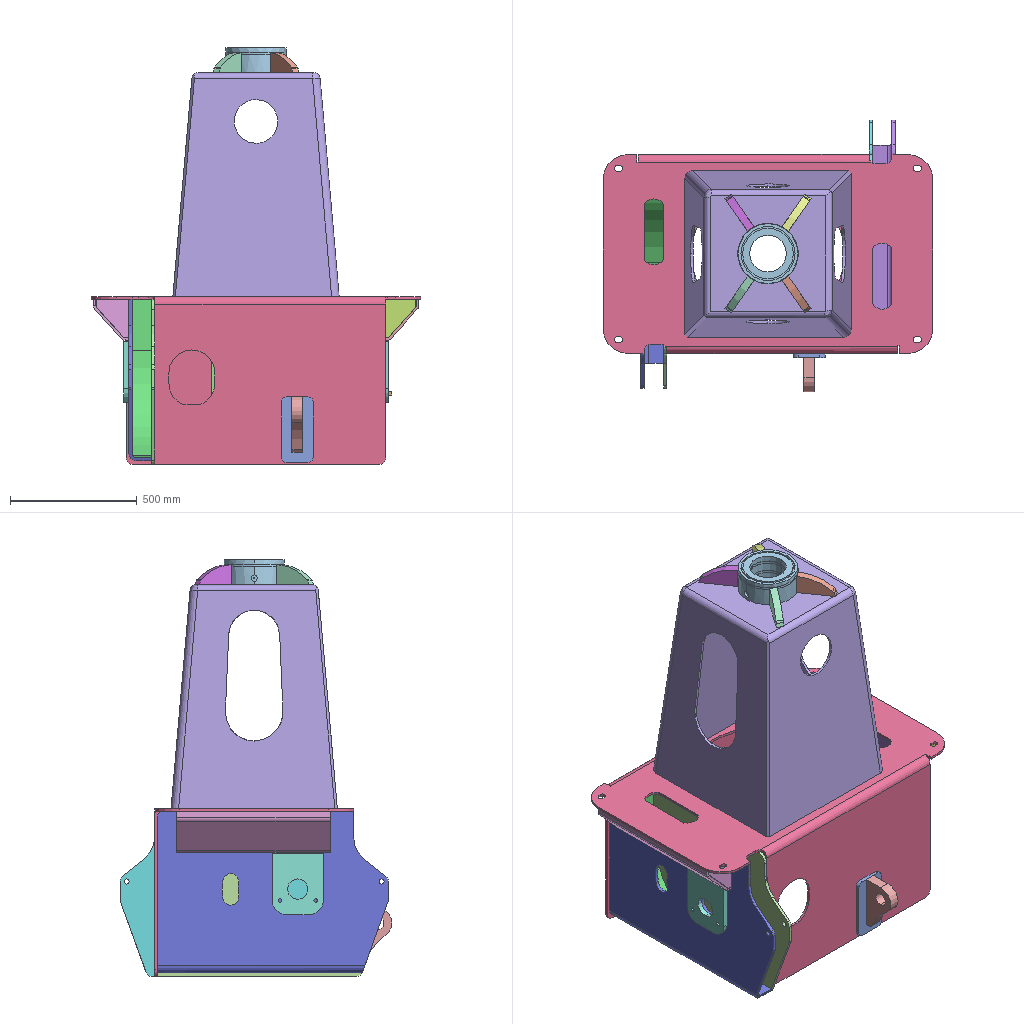Assembly | SolidWorks | 8 different items | 9 placed | box 1300 x 1071 x 1641 mm
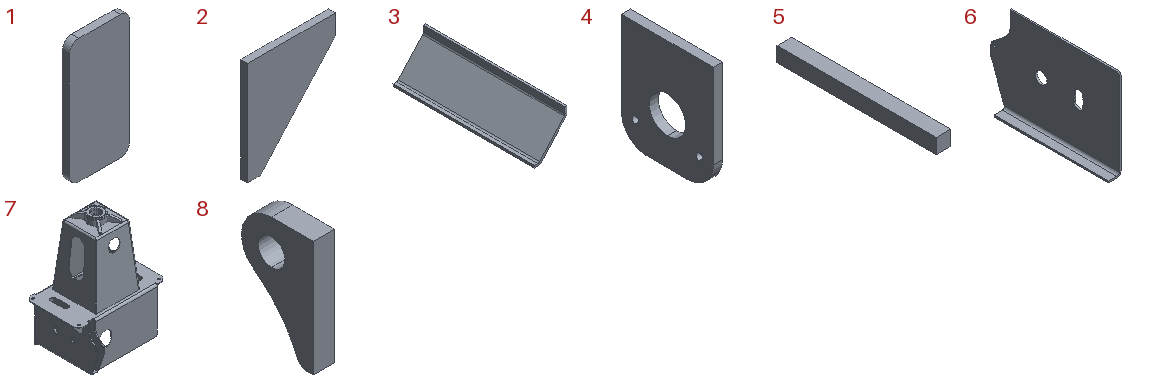Parts list (item | quantity | size | volume | features):
1 | x1 | 126 x 15 x 258.5 mm | 483415 mm3 | features DeleteBody 1, MBimport 1
2 | x1 | 129 x 10 x 152 mm | 128824 mm3 | features DeleteBody 1, MBimport 1
3 | x1 | 140 x 605 x 163 mm | 1343139 mm3 | features DelFace 1, DeleteBody 1, FlatPattern 1, FlattenBends 1, MBimport 1, ProcessBends 1, SheetMetal 1
4 | x2 | 20 x 202 x 242 mm | 844072 mm3 | features DeleteBody 1, MBimport 1
5 | x1 | 15 x 160 x 15 mm | 36000 mm3 | features DeleteBody 1, MBimport 1
6 | x1 | 89 x 910.92 x 637.5 mm | 13906050 mm3 | features DeleteBody 1, FlatPattern 1, MBimport 1, SheetMetal 1, SolidToSheetMetal 1
7 | x1 | 1300 x 1057 x 1641 mm | 81137249 mm3 | features DeleteBody 3, MBimport 1
8 | x1 | 40 x 135.266 x 218 mm | 706740 mm3 | features DeleteBody 1, MBimport 1
Mates (type | each side: item.copy, entity, surface, feature):
Concentric | 4.1 face cylinder X01.stp<1> | 7.1 face cylinder X01.stp<1>
Coincident | 4.1 face plane X01.stp<1> | 7.1 face plane X01.stp<1>
Parallel | 4.1 face plane X01.stp<1> | 7.1 face plane X01.stp<1>
Concentric | 7.1 face cylinder X01.stp<1> | 4.2 face cylinder X01.stp<1>
Parallel | 4.1 face plane X01.stp<1> | 4.2 face plane X01.stp<1>
Coincident | 7.1 face plane X01.stp<1> | 4.2 face plane X01.stp<1>
Coincident | 1.1 face plane X01.stp<1> | 7.1 face plane X01.stp<1> | 2 times
Width | 1.1 face plane X01.stp<1> | 1.1 face plane X01.stp<1> | 7.1 face plane X01.stp<1> | 7.1 face plane X01.stp<1>
Coincident | 8.1 face plane X01.stp<1> | 1.1 face plane X01.stp<1> | 2 times
Width | 8.1 face plane X01.stp<1> | 8.1 face plane X01.stp<1> | 1.1 face plane X01.stp<1> | 1.1 face plane X01.stp<1>
Coincident | 4.1 face plane X01.stp<1> | 5.1 face plane X01.stp<1>
DistanceDim | 4.1 face plane X01.stp<1> | 5.1 face plane X01.stp<1>
Width | 5.1 face plane X01.stp<1> | 5.1 face plane X01.stp<1> | 4.1 face plane X01.stp<1> | 4.1 face plane X01.stp<1>
Coincident | 3.1 face plane X01.stp<1> | 7.1 face plane X01.stp<1> | 3 times
Coincident | 2.1 face plane X01.stp<1> | 7.1 face plane X01.stp<1> | 2 times
Coincident | 2.1 face plane X01.stp<1> | 3.1 face plane X01.stp<1>